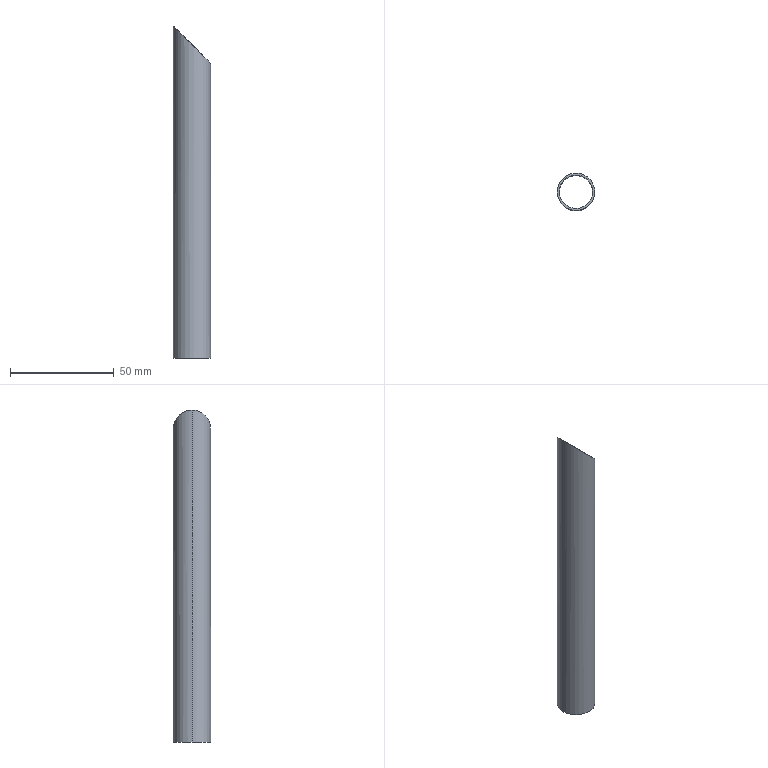Part | SolidWorks | features Extrusion 1, ICE 1 | 1 solid | 6 faces | box 18 x 18 x 160 mm | volume 8065 mm3 | cylinder 4 | plane 2 | commonest cylinder face diameters 16 x2 18 x2
STEP:
#1=CARTESIAN_POINT('',(8.,0.,143.));
#2=VERTEX_POINT('',#1);
#3=CARTESIAN_POINT('',(-8.,0.,159.));
#4=VERTEX_POINT('',#3);
#5=CARTESIAN_POINT('',(8.,0.,143.));
#6=CARTESIAN_POINT('',(8.,-16.,143.));
#7=CARTESIAN_POINT('',(-8.,-16.,159.));
#8=CARTESIAN_POINT('',(-8.,0.,159.));
#9=(BOUNDED_CURVE()B_SPLINE_CURVE(3,(#5,#6,#7,#8),.UNSPECIFIED.,.F.,.F.)B_SPLINE_CURVE_WITH_KNOTS((4,4),(0.,3.142),.UNSPECIFIED.)CURVE()GEOMETRIC_REPRESENTATION_ITEM()RATIONAL_B_SPLINE_CURVE((1.,0.3333,0.3333,1.))REPRESENTATION_ITEM(''));
#10=EDGE_CURVE('',#2,#4,#9,.T.);
#11=ORIENTED_EDGE('',*,*,#10,.F.);
#12=CARTESIAN_POINT('',(8.,0.,0.));
#13=VERTEX_POINT('',#12);
#14=CARTESIAN_POINT('',(8.,0.,160.));
#15=DIRECTION('',(0.,0.,-1.));
#16=VECTOR('',#15,1000.);
#17=LINE('',#14,#16);
#18=EDGE_CURVE('',#2,#13,#17,.T.);
#19=ORIENTED_EDGE('',*,*,#18,.T.);
#20=CARTESIAN_POINT('',(-8.,0.,0.));
#21=VERTEX_POINT('',#20);
#22=CARTESIAN_POINT('',(0.,0.,0.));
#23=DIRECTION('',(0.,0.,1.));
#24=DIRECTION('',(1.,0.,0.));
#25=AXIS2_PLACEMENT_3D('',#22,#23,#24);
#26=CIRCLE('',#25,8.);
#27=EDGE_CURVE('',#21,#13,#26,.T.);
#28=ORIENTED_EDGE('',*,*,#27,.F.);
#29=CARTESIAN_POINT('',(-8.,0.,160.));
#30=DIRECTION('',(0.,0.,-1.));
#31=VECTOR('',#30,1000.);
#32=LINE('',#29,#31);
#33=EDGE_CURVE('',#4,#21,#32,.T.);
#34=ORIENTED_EDGE('',*,*,#33,.F.);
#35=EDGE_LOOP('',(#11,#19,#28,#34));
#36=FACE_OUTER_BOUND('',#35,.T.);
#37=CARTESIAN_POINT('',(0.,0.,160.));
#38=DIRECTION('',(0.,0.,-1.));
#39=DIRECTION('',(-1.,0.,0.));
#40=AXIS2_PLACEMENT_3D('',#37,#38,#39);
#41=CYLINDRICAL_SURFACE('',#40,8.);
#42=ADVANCED_FACE('',(#36),#41,.F.);
#43=CARTESIAN_POINT('',(-9.,0.,160.));
#44=VERTEX_POINT('',#43);
#45=CARTESIAN_POINT('',(9.,0.,142.));
#46=VERTEX_POINT('',#45);
#47=CARTESIAN_POINT('',(-9.,0.,160.));
#48=CARTESIAN_POINT('',(-9.,18.,160.));
#49=CARTESIAN_POINT('',(9.,18.,142.));
#50=CARTESIAN_POINT('',(9.,0.,142.));
#51=(BOUNDED_CURVE()B_SPLINE_CURVE(3,(#47,#48,#49,#50),.UNSPECIFIED.,.F.,.F.)B_SPLINE_CURVE_WITH_KNOTS((4,4),(3.142,6.283),.UNSPECIFIED.)CURVE()GEOMETRIC_REPRESENTATION_ITEM()RATIONAL_B_SPLINE_CURVE((1.,0.3333,0.3333,1.))REPRESENTATION_ITEM(''));
#52=EDGE_CURVE('',#44,#46,#51,.T.);
#53=ORIENTED_EDGE('',*,*,#52,.T.);
#54=CARTESIAN_POINT('',(9.,0.,0.));
#55=VERTEX_POINT('',#54);
#56=CARTESIAN_POINT('',(9.,0.,160.));
#57=DIRECTION('',(0.,0.,-1.));
#58=VECTOR('',#57,1000.);
#59=LINE('',#56,#58);
#60=EDGE_CURVE('',#46,#55,#59,.T.);
#61=ORIENTED_EDGE('',*,*,#60,.T.);
#62=CARTESIAN_POINT('',(-9.,0.,0.));
#63=VERTEX_POINT('',#62);
#64=CARTESIAN_POINT('',(0.,0.,0.));
#65=DIRECTION('',(0.,0.,1.));
#66=DIRECTION('',(1.,0.,0.));
#67=AXIS2_PLACEMENT_3D('',#64,#65,#66);
#68=CIRCLE('',#67,9.);
#69=EDGE_CURVE('',#55,#63,#68,.T.);
#70=ORIENTED_EDGE('',*,*,#69,.T.);
#71=CARTESIAN_POINT('',(-9.,0.,160.));
#72=DIRECTION('',(0.,0.,-1.));
#73=VECTOR('',#72,1000.);
#74=LINE('',#71,#73);
#75=EDGE_CURVE('',#44,#63,#74,.T.);
#76=ORIENTED_EDGE('',*,*,#75,.F.);
#77=EDGE_LOOP('',(#53,#61,#70,#76));
#78=FACE_OUTER_BOUND('',#77,.T.);
#79=CARTESIAN_POINT('',(0.,0.,160.));
#80=DIRECTION('',(0.,0.,-1.));
#81=DIRECTION('',(-1.,0.,0.));
#82=AXIS2_PLACEMENT_3D('',#79,#80,#81);
#83=CYLINDRICAL_SURFACE('',#82,9.);
#84=ADVANCED_FACE('',(#78),#83,.T.);
#85=CARTESIAN_POINT('',(0.,0.,0.));
#86=DIRECTION('',(0.,0.,1.));
#87=DIRECTION('',(1.,0.,0.));
#88=AXIS2_PLACEMENT_3D('',#85,#86,#87);
#89=CIRCLE('',#88,9.);
#90=EDGE_CURVE('',#63,#55,#89,.T.);
#91=ORIENTED_EDGE('',*,*,#90,.F.);
#92=ORIENTED_EDGE('',*,*,#69,.F.);
#93=EDGE_LOOP('',(#91,#92));
#94=FACE_OUTER_BOUND('',#93,.T.);
#95=ORIENTED_EDGE('',*,*,#27,.T.);
#96=CARTESIAN_POINT('',(0.,0.,0.));
#97=DIRECTION('',(0.,0.,1.));
#98=DIRECTION('',(1.,0.,0.));
#99=AXIS2_PLACEMENT_3D('',#96,#97,#98);
#100=CIRCLE('',#99,8.);
#101=EDGE_CURVE('',#13,#21,#100,.T.);
#102=ORIENTED_EDGE('',*,*,#101,.T.);
#103=EDGE_LOOP('',(#95,#102));
#104=FACE_BOUND('',#103,.T.);
#105=CARTESIAN_POINT('',(0.,0.,0.));
#106=DIRECTION('',(0.,0.,1.));
#107=DIRECTION('',(1.,0.,0.));
#108=AXIS2_PLACEMENT_3D('',#105,#106,#107);
#109=PLANE('',#108);
#110=ADVANCED_FACE('',(#94,#104),#109,.F.);
#111=ORIENTED_EDGE('',*,*,#60,.F.);
#112=CARTESIAN_POINT('',(9.,0.,142.));
#113=CARTESIAN_POINT('',(9.,-18.,142.));
#114=CARTESIAN_POINT('',(-9.,-18.,160.));
#115=CARTESIAN_POINT('',(-9.,0.,160.));
#116=(BOUNDED_CURVE()B_SPLINE_CURVE(3,(#112,#113,#114,#115),.UNSPECIFIED.,.F.,.F.)B_SPLINE_CURVE_WITH_KNOTS((4,4),(0.,3.142),.UNSPECIFIED.)CURVE()GEOMETRIC_REPRESENTATION_ITEM()RATIONAL_B_SPLINE_CURVE((1.,0.3333,0.3333,1.))REPRESENTATION_ITEM(''));
#117=EDGE_CURVE('',#46,#44,#116,.T.);
#118=ORIENTED_EDGE('',*,*,#117,.T.);
#119=ORIENTED_EDGE('',*,*,#75,.T.);
#120=ORIENTED_EDGE('',*,*,#90,.T.);
#121=EDGE_LOOP('',(#111,#118,#119,#120));
#122=FACE_OUTER_BOUND('',#121,.T.);
#123=CARTESIAN_POINT('',(0.,0.,160.));
#124=DIRECTION('',(0.,0.,-1.));
#125=DIRECTION('',(-1.,0.,0.));
#126=AXIS2_PLACEMENT_3D('',#123,#124,#125);
#127=CYLINDRICAL_SURFACE('',#126,9.);
#128=ADVANCED_FACE('',(#122),#127,.T.);
#129=ORIENTED_EDGE('',*,*,#18,.F.);
#130=CARTESIAN_POINT('',(-8.,0.,159.));
#131=CARTESIAN_POINT('',(-8.,16.,159.));
#132=CARTESIAN_POINT('',(8.,16.,143.));
#133=CARTESIAN_POINT('',(8.,0.,143.));
#134=(BOUNDED_CURVE()B_SPLINE_CURVE(3,(#130,#131,#132,#133),.UNSPECIFIED.,.F.,.F.)B_SPLINE_CURVE_WITH_KNOTS((4,4),(3.142,6.283),.UNSPECIFIED.)CURVE()GEOMETRIC_REPRESENTATION_ITEM()RATIONAL_B_SPLINE_CURVE((1.,0.3333,0.3333,1.))REPRESENTATION_ITEM(''));
#135=EDGE_CURVE('',#4,#2,#134,.T.);
#136=ORIENTED_EDGE('',*,*,#135,.F.);
#137=ORIENTED_EDGE('',*,*,#33,.T.);
#138=ORIENTED_EDGE('',*,*,#101,.F.);
#139=EDGE_LOOP('',(#129,#136,#137,#138));
#140=FACE_OUTER_BOUND('',#139,.T.);
#141=CARTESIAN_POINT('',(0.,0.,160.));
#142=DIRECTION('',(0.,0.,-1.));
#143=DIRECTION('',(-1.,0.,0.));
#144=AXIS2_PLACEMENT_3D('',#141,#142,#143);
#145=CYLINDRICAL_SURFACE('',#144,8.);
#146=ADVANCED_FACE('',(#140),#145,.F.);
#147=ORIENTED_EDGE('',*,*,#135,.T.);
#148=ORIENTED_EDGE('',*,*,#10,.T.);
#149=EDGE_LOOP('',(#147,#148));
#150=FACE_BOUND('',#149,.T.);
#151=ORIENTED_EDGE('',*,*,#52,.F.);
#152=ORIENTED_EDGE('',*,*,#117,.F.);
#153=EDGE_LOOP('',(#151,#152));
#154=FACE_OUTER_BOUND('',#153,.T.);
#155=CARTESIAN_POINT('',(-9.,-80.,160.));
#156=DIRECTION('',(-0.7071,0.,-0.7071));
#157=DIRECTION('',(-0.7071,0.,0.7071));
#158=AXIS2_PLACEMENT_3D('',#155,#156,#157);
#159=PLANE('',#158);
#160=ADVANCED_FACE('',(#150,#154),#159,.F.);
#161=CLOSED_SHELL('',(#42,#84,#110,#128,#146,#160));
#162=MANIFOLD_SOLID_BREP('',#161);
#163=CARTESIAN_POINT('',(0.,0.,0.));
#164=DIRECTION('',(0.,0.,1.));
#165=DIRECTION('',(1.,0.,0.));
#166=AXIS2_PLACEMENT_3D('',#163,#164,#165);
#167=(LENGTH_UNIT()NAMED_UNIT(*)SI_UNIT(.MILLI.,.METRE.));
#168=UNCERTAINTY_MEASURE_WITH_UNIT(LENGTH_MEASURE(0.00001),#167,'','');
#169=(NAMED_UNIT(*)PLANE_ANGLE_UNIT()SI_UNIT($,.RADIAN.));
#170=(NAMED_UNIT(*)SI_UNIT($,.STERADIAN.)SOLID_ANGLE_UNIT());
#171=(GEOMETRIC_REPRESENTATION_CONTEXT(3)GLOBAL_UNCERTAINTY_ASSIGNED_CONTEXT((#168))GLOBAL_UNIT_ASSIGNED_CONTEXT((#167,#169,#170))REPRESENTATION_CONTEXT('',''));
#172=ADVANCED_BREP_SHAPE_REPRESENTATION('',(#162,#166),#171);